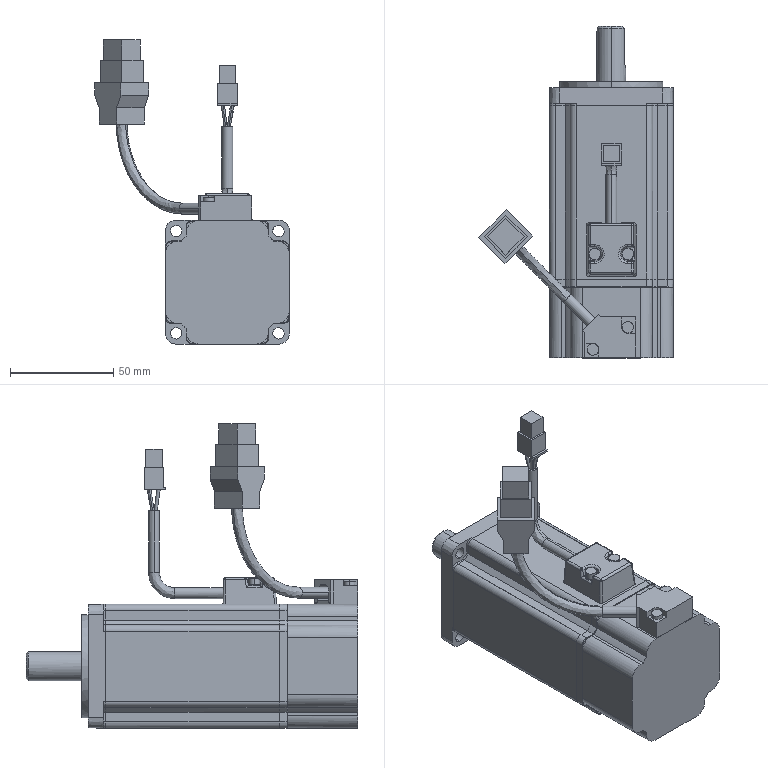Part | SolidWorks | features BaseBody 1 | 1 solid | 415 faces | box 94.241 x 160.703 x 147.367 mm | volume 450542 mm3 | plane 189 | cylinder 163 | spline 37 | cone 26 | commonest cylinder face diameters 6 x41 2 x20 5.5 x16 0.6 x12 1.5 x11 5.3 x8